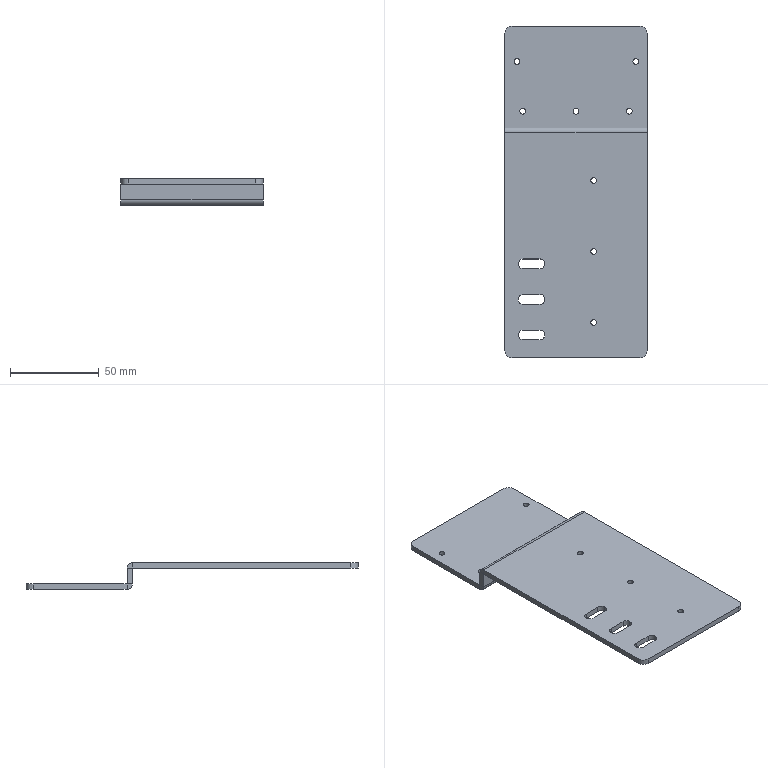Part | STEP file | 1 solid | 57 faces | box 80 x 187 x 15 mm | volume 46500 mm3 | cylinder 33 | plane 24 | commonest cylinder face diameters 3.3 x16 5.5 x9 8 x4 0.2 x2 6.2 x2